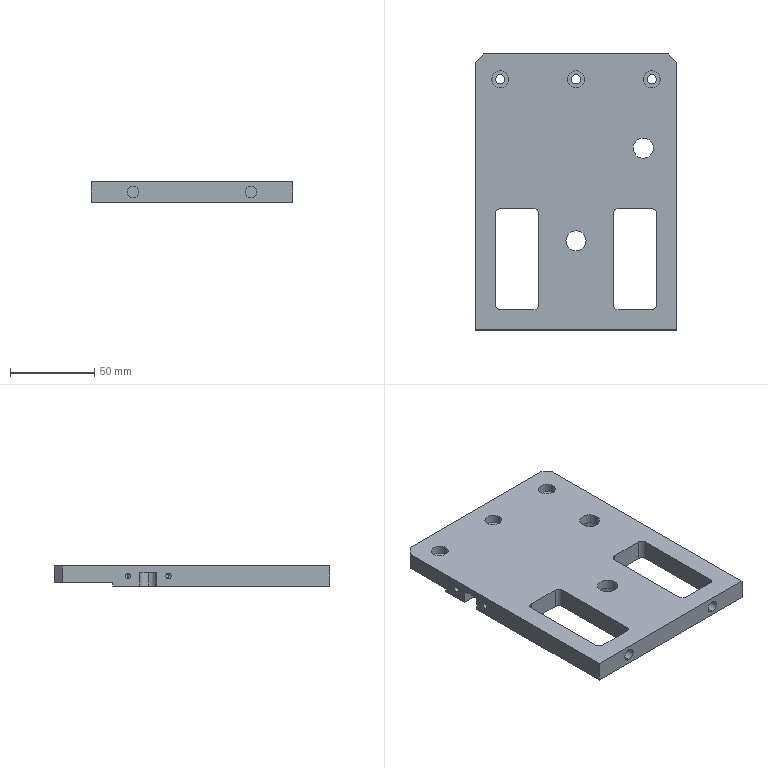Part | STEP file | Conveyor Line Bracket-Mirror | 1 solid | 68 faces | box 120 x 164 x 12 mm | volume 177189 mm3 | cylinder 38 | plane 26 | cone 4 | commonest cylinder face diameters 6 x8 10 x8 5.5 x6 3.3 x4 7 x4 12 x4